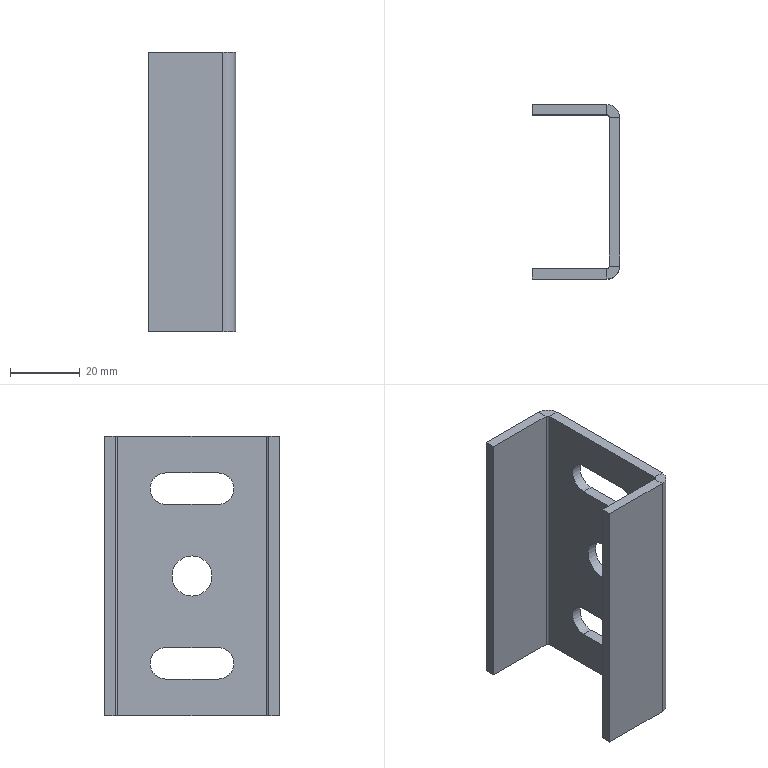Part | SolidWorks | features EdgeFlange 1, FlatPattern 1, SMBaseFlange 1, SheetMetal 1 | 1 solid | 32 faces | box 25 x 50 x 80 mm | volume 20596 mm3 | plane 22 | cylinder 10 | commonest cylinder face diameters 9 x4 1.473 x2 7.473 x2 11.5 x2
STEP:
#1=CARTESIAN_POINT('',(-3.,-25.,-34.25));
#2=VERTEX_POINT('',#1);
#3=CARTESIAN_POINT('',(-3.,-25.,-45.75));
#4=VERTEX_POINT('',#3);
#5=CARTESIAN_POINT('',(-3.,-25.,-40.));
#6=DIRECTION('',(1.,0.,0.));
#7=DIRECTION('',(0.,0.,-1.));
#8=AXIS2_PLACEMENT_3D('',#5,#6,#7);
#9=CIRCLE('',#8,5.75);
#10=EDGE_CURVE('',#2,#4,#9,.T.);
#11=ORIENTED_EDGE('',*,*,#10,.F.);
#12=CARTESIAN_POINT('',(0.,-25.,-34.25));
#13=VERTEX_POINT('',#12);
#14=CARTESIAN_POINT('',(-3.,-25.,-34.25));
#15=DIRECTION('',(1.,0.,0.));
#16=VECTOR('',#15,1000.);
#17=LINE('',#14,#16);
#18=EDGE_CURVE('',#2,#13,#17,.T.);
#19=ORIENTED_EDGE('',*,*,#18,.T.);
#20=CARTESIAN_POINT('',(0.,-25.,-45.75));
#21=VERTEX_POINT('',#20);
#22=CARTESIAN_POINT('',(0.,-25.,-40.));
#23=DIRECTION('',(1.,0.,0.));
#24=DIRECTION('',(0.,0.,-1.));
#25=AXIS2_PLACEMENT_3D('',#22,#23,#24);
#26=CIRCLE('',#25,5.75);
#27=EDGE_CURVE('',#13,#21,#26,.T.);
#28=ORIENTED_EDGE('',*,*,#27,.T.);
#29=CARTESIAN_POINT('',(-3.,-25.,-45.75));
#30=DIRECTION('',(1.,0.,0.));
#31=VECTOR('',#30,1000.);
#32=LINE('',#29,#31);
#33=EDGE_CURVE('',#4,#21,#32,.T.);
#34=ORIENTED_EDGE('',*,*,#33,.F.);
#35=EDGE_LOOP('',(#11,#19,#28,#34));
#36=FACE_OUTER_BOUND('',#35,.T.);
#37=CARTESIAN_POINT('',(-3.,-25.,-40.));
#38=DIRECTION('',(1.,0.,0.));
#39=DIRECTION('',(0.,0.,-1.));
#40=AXIS2_PLACEMENT_3D('',#37,#38,#39);
#41=CYLINDRICAL_SURFACE('',#40,5.75);
#42=ADVANCED_FACE('',(#36),#41,.F.);
#43=CARTESIAN_POINT('',(-3.,-32.5,-69.5));
#44=VERTEX_POINT('',#43);
#45=CARTESIAN_POINT('',(-3.,-17.5,-69.5));
#46=VERTEX_POINT('',#45);
#47=CARTESIAN_POINT('',(-3.,-17.5,-69.5));
#48=DIRECTION('',(0.,1.,0.));
#49=VECTOR('',#48,1000.);
#50=LINE('',#47,#49);
#51=EDGE_CURVE('',#44,#46,#50,.T.);
#52=ORIENTED_EDGE('',*,*,#51,.T.);
#53=CARTESIAN_POINT('',(-3.,-17.5,-60.5));
#54=VERTEX_POINT('',#53);
#55=CARTESIAN_POINT('',(-3.,-17.5,-65.));
#56=DIRECTION('',(1.,0.,0.));
#57=DIRECTION('',(0.,0.,-1.));
#58=AXIS2_PLACEMENT_3D('',#55,#56,#57);
#59=CIRCLE('',#58,4.5);
#60=EDGE_CURVE('',#46,#54,#59,.T.);
#61=ORIENTED_EDGE('',*,*,#60,.T.);
#62=CARTESIAN_POINT('',(-3.,-32.5,-60.5));
#63=VERTEX_POINT('',#62);
#64=CARTESIAN_POINT('',(-3.,-17.5,-60.5));
#65=DIRECTION('',(0.,-1.,0.));
#66=VECTOR('',#65,1000.);
#67=LINE('',#64,#66);
#68=EDGE_CURVE('',#54,#63,#67,.T.);
#69=ORIENTED_EDGE('',*,*,#68,.T.);
#70=CARTESIAN_POINT('',(-3.,-32.5,-65.));
#71=DIRECTION('',(1.,0.,0.));
#72=DIRECTION('',(0.,0.,-1.));
#73=AXIS2_PLACEMENT_3D('',#70,#71,#72);
#74=CIRCLE('',#73,4.5);
#75=EDGE_CURVE('',#63,#44,#74,.T.);
#76=ORIENTED_EDGE('',*,*,#75,.T.);
#77=EDGE_LOOP('',(#52,#61,#69,#76));
#78=FACE_BOUND('',#77,.T.);
#79=CARTESIAN_POINT('',(-3.,-32.5,-19.5));
#80=VERTEX_POINT('',#79);
#81=CARTESIAN_POINT('',(-3.,-17.5,-19.5));
#82=VERTEX_POINT('',#81);
#83=CARTESIAN_POINT('',(-3.,-17.5,-19.5));
#84=DIRECTION('',(0.,1.,0.));
#85=VECTOR('',#84,1000.);
#86=LINE('',#83,#85);
#87=EDGE_CURVE('',#80,#82,#86,.T.);
#88=ORIENTED_EDGE('',*,*,#87,.T.);
#89=CARTESIAN_POINT('',(-3.,-17.5,-10.5));
#90=VERTEX_POINT('',#89);
#91=CARTESIAN_POINT('',(-3.,-17.5,-15.));
#92=DIRECTION('',(1.,0.,0.));
#93=DIRECTION('',(0.,0.,-1.));
#94=AXIS2_PLACEMENT_3D('',#91,#92,#93);
#95=CIRCLE('',#94,4.5);
#96=EDGE_CURVE('',#82,#90,#95,.T.);
#97=ORIENTED_EDGE('',*,*,#96,.T.);
#98=CARTESIAN_POINT('',(-3.,-32.5,-10.5));
#99=VERTEX_POINT('',#98);
#100=CARTESIAN_POINT('',(-3.,-17.5,-10.5));
#101=DIRECTION('',(0.,-1.,0.));
#102=VECTOR('',#101,1000.);
#103=LINE('',#100,#102);
#104=EDGE_CURVE('',#90,#99,#103,.T.);
#105=ORIENTED_EDGE('',*,*,#104,.T.);
#106=CARTESIAN_POINT('',(-3.,-32.5,-15.));
#107=DIRECTION('',(1.,0.,0.));
#108=DIRECTION('',(0.,0.,-1.));
#109=AXIS2_PLACEMENT_3D('',#106,#107,#108);
#110=CIRCLE('',#109,4.5);
#111=EDGE_CURVE('',#99,#80,#110,.T.);
#112=ORIENTED_EDGE('',*,*,#111,.T.);
#113=EDGE_LOOP('',(#88,#97,#105,#112));
#114=FACE_BOUND('',#113,.T.);
#115=CARTESIAN_POINT('',(-3.,-25.,-40.));
#116=DIRECTION('',(1.,0.,0.));
#117=DIRECTION('',(0.,0.,-1.));
#118=AXIS2_PLACEMENT_3D('',#115,#116,#117);
#119=CIRCLE('',#118,5.75);
#120=EDGE_CURVE('',#4,#2,#119,.T.);
#121=ORIENTED_EDGE('',*,*,#120,.T.);
#122=ORIENTED_EDGE('',*,*,#10,.T.);
#123=EDGE_LOOP('',(#121,#122));
#124=FACE_BOUND('',#123,.T.);
#125=CARTESIAN_POINT('',(-3.,-46.263,0.));
#126=VERTEX_POINT('',#125);
#127=CARTESIAN_POINT('',(-3.,-46.263,-80.));
#128=VERTEX_POINT('',#127);
#129=CARTESIAN_POINT('',(-3.,-46.263,0.));
#130=DIRECTION('',(0.,0.,-1.));
#131=VECTOR('',#130,1000.);
#132=LINE('',#129,#131);
#133=EDGE_CURVE('',#126,#128,#132,.T.);
#134=ORIENTED_EDGE('',*,*,#133,.F.);
#135=CARTESIAN_POINT('',(-3.,-3.737,0.));
#136=VERTEX_POINT('',#135);
#137=CARTESIAN_POINT('',(-3.,0.,0.));
#138=DIRECTION('',(0.,-1.,0.));
#139=VECTOR('',#138,1000.);
#140=LINE('',#137,#139);
#141=EDGE_CURVE('',#136,#126,#140,.T.);
#142=ORIENTED_EDGE('',*,*,#141,.F.);
#143=CARTESIAN_POINT('',(-3.,-3.737,-80.));
#144=VERTEX_POINT('',#143);
#145=CARTESIAN_POINT('',(-3.,-3.737,-80.));
#146=DIRECTION('',(0.,0.,1.));
#147=VECTOR('',#146,1000.);
#148=LINE('',#145,#147);
#149=EDGE_CURVE('',#144,#136,#148,.T.);
#150=ORIENTED_EDGE('',*,*,#149,.F.);
#151=CARTESIAN_POINT('',(-3.,0.,-80.));
#152=DIRECTION('',(0.,1.,0.));
#153=VECTOR('',#152,1000.);
#154=LINE('',#151,#153);
#155=EDGE_CURVE('',#128,#144,#154,.T.);
#156=ORIENTED_EDGE('',*,*,#155,.F.);
#157=EDGE_LOOP('',(#134,#142,#150,#156));
#158=FACE_OUTER_BOUND('',#157,.T.);
#159=CARTESIAN_POINT('',(-3.,0.,0.));
#160=DIRECTION('',(1.,0.,0.));
#161=DIRECTION('',(0.,0.,-1.));
#162=AXIS2_PLACEMENT_3D('',#159,#160,#161);
#163=PLANE('',#162);
#164=ADVANCED_FACE('',(#78,#114,#124,#158),#163,.F.);
#165=CARTESIAN_POINT('',(0.,-17.5,-69.5));
#166=VERTEX_POINT('',#165);
#167=CARTESIAN_POINT('',(0.,-17.5,-60.5));
#168=VERTEX_POINT('',#167);
#169=CARTESIAN_POINT('',(0.,-17.5,-65.));
#170=DIRECTION('',(1.,0.,0.));
#171=DIRECTION('',(0.,0.,-1.));
#172=AXIS2_PLACEMENT_3D('',#169,#170,#171);
#173=CIRCLE('',#172,4.5);
#174=EDGE_CURVE('',#166,#168,#173,.T.);
#175=ORIENTED_EDGE('',*,*,#174,.F.);
#176=CARTESIAN_POINT('',(0.,-32.5,-69.5));
#177=VERTEX_POINT('',#176);
#178=CARTESIAN_POINT('',(0.,-17.5,-69.5));
#179=DIRECTION('',(0.,1.,0.));
#180=VECTOR('',#179,1000.);
#181=LINE('',#178,#180);
#182=EDGE_CURVE('',#177,#166,#181,.T.);
#183=ORIENTED_EDGE('',*,*,#182,.F.);
#184=CARTESIAN_POINT('',(0.,-32.5,-60.5));
#185=VERTEX_POINT('',#184);
#186=CARTESIAN_POINT('',(0.,-32.5,-65.));
#187=DIRECTION('',(1.,0.,0.));
#188=DIRECTION('',(0.,0.,-1.));
#189=AXIS2_PLACEMENT_3D('',#186,#187,#188);
#190=CIRCLE('',#189,4.5);
#191=EDGE_CURVE('',#185,#177,#190,.T.);
#192=ORIENTED_EDGE('',*,*,#191,.F.);
#193=CARTESIAN_POINT('',(0.,-17.5,-60.5));
#194=DIRECTION('',(0.,-1.,0.));
#195=VECTOR('',#194,1000.);
#196=LINE('',#193,#195);
#197=EDGE_CURVE('',#168,#185,#196,.T.);
#198=ORIENTED_EDGE('',*,*,#197,.F.);
#199=EDGE_LOOP('',(#175,#183,#192,#198));
#200=FACE_BOUND('',#199,.T.);
#201=CARTESIAN_POINT('',(0.,-17.5,-19.5));
#202=VERTEX_POINT('',#201);
#203=CARTESIAN_POINT('',(0.,-17.5,-10.5));
#204=VERTEX_POINT('',#203);
#205=CARTESIAN_POINT('',(0.,-17.5,-15.));
#206=DIRECTION('',(1.,0.,0.));
#207=DIRECTION('',(0.,0.,-1.));
#208=AXIS2_PLACEMENT_3D('',#205,#206,#207);
#209=CIRCLE('',#208,4.5);
#210=EDGE_CURVE('',#202,#204,#209,.T.);
#211=ORIENTED_EDGE('',*,*,#210,.F.);
#212=CARTESIAN_POINT('',(0.,-32.5,-19.5));
#213=VERTEX_POINT('',#212);
#214=CARTESIAN_POINT('',(0.,-17.5,-19.5));
#215=DIRECTION('',(0.,1.,0.));
#216=VECTOR('',#215,1000.);
#217=LINE('',#214,#216);
#218=EDGE_CURVE('',#213,#202,#217,.T.);
#219=ORIENTED_EDGE('',*,*,#218,.F.);
#220=CARTESIAN_POINT('',(0.,-32.5,-10.5));
#221=VERTEX_POINT('',#220);
#222=CARTESIAN_POINT('',(0.,-32.5,-15.));
#223=DIRECTION('',(1.,0.,0.));
#224=DIRECTION('',(0.,0.,-1.));
#225=AXIS2_PLACEMENT_3D('',#222,#223,#224);
#226=CIRCLE('',#225,4.5);
#227=EDGE_CURVE('',#221,#213,#226,.T.);
#228=ORIENTED_EDGE('',*,*,#227,.F.);
#229=CARTESIAN_POINT('',(0.,-17.5,-10.5));
#230=DIRECTION('',(0.,-1.,0.));
#231=VECTOR('',#230,1000.);
#232=LINE('',#229,#231);
#233=EDGE_CURVE('',#204,#221,#232,.T.);
#234=ORIENTED_EDGE('',*,*,#233,.F.);
#235=EDGE_LOOP('',(#211,#219,#228,#234));
#236=FACE_BOUND('',#235,.T.);
#237=CARTESIAN_POINT('',(0.,-25.,-40.));
#238=DIRECTION('',(1.,0.,0.));
#239=DIRECTION('',(0.,0.,-1.));
#240=AXIS2_PLACEMENT_3D('',#237,#238,#239);
#241=CIRCLE('',#240,5.75);
#242=EDGE_CURVE('',#21,#13,#241,.T.);
#243=ORIENTED_EDGE('',*,*,#242,.F.);
#244=ORIENTED_EDGE('',*,*,#27,.F.);
#245=EDGE_LOOP('',(#243,#244));
#246=FACE_BOUND('',#245,.T.);
#247=CARTESIAN_POINT('',(0.,-3.737,0.));
#248=VERTEX_POINT('',#247);
#249=CARTESIAN_POINT('',(0.,-46.263,0.));
#250=VERTEX_POINT('',#249);
#251=CARTESIAN_POINT('',(0.,0.,0.));
#252=DIRECTION('',(0.,-1.,0.));
#253=VECTOR('',#252,1000.);
#254=LINE('',#251,#253);
#255=EDGE_CURVE('',#248,#250,#254,.T.);
#256=ORIENTED_EDGE('',*,*,#255,.T.);
#257=CARTESIAN_POINT('',(0.,-46.263,-80.));
#258=VERTEX_POINT('',#257);
#259=CARTESIAN_POINT('',(0.,-46.263,0.));
#260=DIRECTION('',(0.,0.,-1.));
#261=VECTOR('',#260,1000.);
#262=LINE('',#259,#261);
#263=EDGE_CURVE('',#250,#258,#262,.T.);
#264=ORIENTED_EDGE('',*,*,#263,.T.);
#265=CARTESIAN_POINT('',(0.,-3.737,-80.));
#266=VERTEX_POINT('',#265);
#267=CARTESIAN_POINT('',(0.,0.,-80.));
#268=DIRECTION('',(0.,1.,0.));
#269=VECTOR('',#268,1000.);
#270=LINE('',#267,#269);
#271=EDGE_CURVE('',#258,#266,#270,.T.);
#272=ORIENTED_EDGE('',*,*,#271,.T.);
#273=CARTESIAN_POINT('',(0.,-3.737,-80.));
#274=DIRECTION('',(0.,0.,1.));
#275=VECTOR('',#274,1000.);
#276=LINE('',#273,#275);
#277=EDGE_CURVE('',#266,#248,#276,.T.);
#278=ORIENTED_EDGE('',*,*,#277,.T.);
#279=EDGE_LOOP('',(#256,#264,#272,#278));
#280=FACE_OUTER_BOUND('',#279,.T.);
#281=CARTESIAN_POINT('',(0.,0.,0.));
#282=DIRECTION('',(1.,0.,0.));
#283=DIRECTION('',(0.,0.,-1.));
#284=AXIS2_PLACEMENT_3D('',#281,#282,#283);
#285=PLANE('',#284);
#286=ADVANCED_FACE('',(#200,#236,#246,#280),#285,.T.);
#287=ORIENTED_EDGE('',*,*,#141,.T.);
#288=CARTESIAN_POINT('',(-3.,-46.263,0.));
#289=DIRECTION('',(1.,0.,0.));
#290=VECTOR('',#289,1000.);
#291=LINE('',#288,#290);
#292=EDGE_CURVE('',#126,#250,#291,.T.);
#293=ORIENTED_EDGE('',*,*,#292,.T.);
#294=ORIENTED_EDGE('',*,*,#255,.F.);
#295=CARTESIAN_POINT('',(-3.,-3.737,0.));
#296=DIRECTION('',(1.,0.,0.));
#297=VECTOR('',#296,1000.);
#298=LINE('',#295,#297);
#299=EDGE_CURVE('',#136,#248,#298,.T.);
#300=ORIENTED_EDGE('',*,*,#299,.F.);
#301=EDGE_LOOP('',(#287,#293,#294,#300));
#302=FACE_OUTER_BOUND('',#301,.T.);
#303=CARTESIAN_POINT('',(-3.,0.,0.));
#304=DIRECTION('',(0.,0.,1.));
#305=DIRECTION('',(0.,-1.,0.));
#306=AXIS2_PLACEMENT_3D('',#303,#304,#305);
#307=PLANE('',#306);
#308=ADVANCED_FACE('',(#302),#307,.T.);
#309=CARTESIAN_POINT('',(-3.,-46.263,-80.));
#310=DIRECTION('',(1.,0.,0.));
#311=VECTOR('',#310,1000.);
#312=LINE('',#309,#311);
#313=EDGE_CURVE('',#128,#258,#312,.T.);
#314=ORIENTED_EDGE('',*,*,#313,.F.);
#315=ORIENTED_EDGE('',*,*,#155,.T.);
#316=CARTESIAN_POINT('',(-3.,-3.737,-80.));
#317=DIRECTION('',(1.,0.,0.));
#318=VECTOR('',#317,1000.);
#319=LINE('',#316,#318);
#320=EDGE_CURVE('',#144,#266,#319,.T.);
#321=ORIENTED_EDGE('',*,*,#320,.T.);
#322=ORIENTED_EDGE('',*,*,#271,.F.);
#323=EDGE_LOOP('',(#314,#315,#321,#322));
#324=FACE_OUTER_BOUND('',#323,.T.);
#325=CARTESIAN_POINT('',(-3.,0.,-80.));
#326=DIRECTION('',(0.,0.,-1.));
#327=DIRECTION('',(-1.,0.,0.));
#328=AXIS2_PLACEMENT_3D('',#325,#326,#327);
#329=PLANE('',#328);
#330=ADVANCED_FACE('',(#324),#329,.T.);
#331=ORIENTED_EDGE('',*,*,#18,.F.);
#332=ORIENTED_EDGE('',*,*,#120,.F.);
#333=ORIENTED_EDGE('',*,*,#33,.T.);
#334=ORIENTED_EDGE('',*,*,#242,.T.);
#335=EDGE_LOOP('',(#331,#332,#333,#334));
#336=FACE_OUTER_BOUND('',#335,.T.);
#337=CARTESIAN_POINT('',(-3.,-25.,-40.));
#338=DIRECTION('',(1.,0.,0.));
#339=DIRECTION('',(0.,0.,-1.));
#340=AXIS2_PLACEMENT_3D('',#337,#338,#339);
#341=CYLINDRICAL_SURFACE('',#340,5.75);
#342=ADVANCED_FACE('',(#336),#341,.F.);
#343=ORIENTED_EDGE('',*,*,#210,.T.);
#344=CARTESIAN_POINT('',(-3.,-17.5,-10.5));
#345=DIRECTION('',(1.,0.,0.));
#346=VECTOR('',#345,1000.);
#347=LINE('',#344,#346);
#348=EDGE_CURVE('',#90,#204,#347,.T.);
#349=ORIENTED_EDGE('',*,*,#348,.F.);
#350=ORIENTED_EDGE('',*,*,#96,.F.);
#351=CARTESIAN_POINT('',(-3.,-17.5,-19.5));
#352=DIRECTION('',(1.,0.,0.));
#353=VECTOR('',#352,1000.);
#354=LINE('',#351,#353);
#355=EDGE_CURVE('',#82,#202,#354,.T.);
#356=ORIENTED_EDGE('',*,*,#355,.T.);
#357=EDGE_LOOP('',(#343,#349,#350,#356));
#358=FACE_OUTER_BOUND('',#357,.T.);
#359=CARTESIAN_POINT('',(-3.,-17.5,-15.));
#360=DIRECTION('',(1.,0.,0.));
#361=DIRECTION('',(0.,0.,-1.));
#362=AXIS2_PLACEMENT_3D('',#359,#360,#361);
#363=CYLINDRICAL_SURFACE('',#362,4.5);
#364=ADVANCED_FACE('',(#358),#363,.F.);
#365=ORIENTED_EDGE('',*,*,#218,.T.);
#366=ORIENTED_EDGE('',*,*,#355,.F.);
#367=ORIENTED_EDGE('',*,*,#87,.F.);
#368=CARTESIAN_POINT('',(-3.,-32.5,-19.5));
#369=DIRECTION('',(1.,0.,0.));
#370=VECTOR('',#369,1000.);
#371=LINE('',#368,#370);
#372=EDGE_CURVE('',#80,#213,#371,.T.);
#373=ORIENTED_EDGE('',*,*,#372,.T.);
#374=EDGE_LOOP('',(#365,#366,#367,#373));
#375=FACE_OUTER_BOUND('',#374,.T.);
#376=CARTESIAN_POINT('',(-3.,-17.5,-19.5));
#377=DIRECTION('',(0.,0.,-1.));
#378=DIRECTION('',(-1.,0.,0.));
#379=AXIS2_PLACEMENT_3D('',#376,#377,#378);
#380=PLANE('',#379);
#381=ADVANCED_FACE('',(#375),#380,.F.);
#382=ORIENTED_EDGE('',*,*,#227,.T.);
#383=ORIENTED_EDGE('',*,*,#372,.F.);
#384=ORIENTED_EDGE('',*,*,#111,.F.);
#385=CARTESIAN_POINT('',(-3.,-32.5,-10.5));
#386=DIRECTION('',(1.,0.,0.));
#387=VECTOR('',#386,1000.);
#388=LINE('',#385,#387);
#389=EDGE_CURVE('',#99,#221,#388,.T.);
#390=ORIENTED_EDGE('',*,*,#389,.T.);
#391=EDGE_LOOP('',(#382,#383,#384,#390));
#392=FACE_OUTER_BOUND('',#391,.T.);
#393=CARTESIAN_POINT('',(-3.,-32.5,-15.));
#394=DIRECTION('',(1.,0.,0.));
#395=DIRECTION('',(0.,0.,-1.));
#396=AXIS2_PLACEMENT_3D('',#393,#394,#395);
#397=CYLINDRICAL_SURFACE('',#396,4.5);
#398=ADVANCED_FACE('',(#392),#397,.F.);
#399=ORIENTED_EDGE('',*,*,#233,.T.);
#400=ORIENTED_EDGE('',*,*,#389,.F.);
#401=ORIENTED_EDGE('',*,*,#104,.F.);
#402=ORIENTED_EDGE('',*,*,#348,.T.);
#403=EDGE_LOOP('',(#399,#400,#401,#402));
#404=FACE_OUTER_BOUND('',#403,.T.);
#405=CARTESIAN_POINT('',(-3.,-17.5,-10.5));
#406=DIRECTION('',(0.,0.,1.));
#407=DIRECTION('',(1.,0.,0.));
#408=AXIS2_PLACEMENT_3D('',#405,#406,#407);
#409=PLANE('',#408);
#410=ADVANCED_FACE('',(#404),#409,.F.);
#411=ORIENTED_EDGE('',*,*,#174,.T.);
#412=CARTESIAN_POINT('',(-3.,-17.5,-60.5));
#413=DIRECTION('',(1.,0.,0.));
#414=VECTOR('',#413,1000.);
#415=LINE('',#412,#414);
#416=EDGE_CURVE('',#54,#168,#415,.T.);
#417=ORIENTED_EDGE('',*,*,#416,.F.);
#418=ORIENTED_EDGE('',*,*,#60,.F.);
#419=CARTESIAN_POINT('',(-3.,-17.5,-69.5));
#420=DIRECTION('',(1.,0.,0.));
#421=VECTOR('',#420,1000.);
#422=LINE('',#419,#421);
#423=EDGE_CURVE('',#46,#166,#422,.T.);
#424=ORIENTED_EDGE('',*,*,#423,.T.);
#425=EDGE_LOOP('',(#411,#417,#418,#424));
#426=FACE_OUTER_BOUND('',#425,.T.);
#427=CARTESIAN_POINT('',(-3.,-17.5,-65.));
#428=DIRECTION('',(1.,0.,0.));
#429=DIRECTION('',(0.,0.,-1.));
#430=AXIS2_PLACEMENT_3D('',#427,#428,#429);
#431=CYLINDRICAL_SURFACE('',#430,4.5);
#432=ADVANCED_FACE('',(#426),#431,.F.);
#433=ORIENTED_EDGE('',*,*,#182,.T.);
#434=ORIENTED_EDGE('',*,*,#423,.F.);
#435=ORIENTED_EDGE('',*,*,#51,.F.);
#436=CARTESIAN_POINT('',(-3.,-32.5,-69.5));
#437=DIRECTION('',(1.,0.,0.));
#438=VECTOR('',#437,1000.);
#439=LINE('',#436,#438);
#440=EDGE_CURVE('',#44,#177,#439,.T.);
#441=ORIENTED_EDGE('',*,*,#440,.T.);
#442=EDGE_LOOP('',(#433,#434,#435,#441));
#443=FACE_OUTER_BOUND('',#442,.T.);
#444=CARTESIAN_POINT('',(-3.,-17.5,-69.5));
#445=DIRECTION('',(0.,0.,-1.));
#446=DIRECTION('',(0.,1.,0.));
#447=AXIS2_PLACEMENT_3D('',#444,#445,#446);
#448=PLANE('',#447);
#449=ADVANCED_FACE('',(#443),#448,.F.);
#450=ORIENTED_EDGE('',*,*,#191,.T.);
#451=ORIENTED_EDGE('',*,*,#440,.F.);
#452=ORIENTED_EDGE('',*,*,#75,.F.);
#453=CARTESIAN_POINT('',(-3.,-32.5,-60.5));
#454=DIRECTION('',(1.,0.,0.));
#455=VECTOR('',#454,1000.);
#456=LINE('',#453,#455);
#457=EDGE_CURVE('',#63,#185,#456,.T.);
#458=ORIENTED_EDGE('',*,*,#457,.T.);
#459=EDGE_LOOP('',(#450,#451,#452,#458));
#460=FACE_OUTER_BOUND('',#459,.T.);
#461=CARTESIAN_POINT('',(-3.,-32.5,-65.));
#462=DIRECTION('',(1.,0.,0.));
#463=DIRECTION('',(0.,0.,-1.));
#464=AXIS2_PLACEMENT_3D('',#461,#462,#463);
#465=CYLINDRICAL_SURFACE('',#464,4.5);
#466=ADVANCED_FACE('',(#460),#465,.F.);
#467=ORIENTED_EDGE('',*,*,#197,.T.);
#468=ORIENTED_EDGE('',*,*,#457,.F.);
#469=ORIENTED_EDGE('',*,*,#68,.F.);
#470=ORIENTED_EDGE('',*,*,#416,.T.);
#471=EDGE_LOOP('',(#467,#468,#469,#470));
#472=FACE_OUTER_BOUND('',#471,.T.);
#473=CARTESIAN_POINT('',(-3.,-17.5,-60.5));
#474=DIRECTION('',(0.,0.,1.));
#475=DIRECTION('',(0.,-1.,0.));
#476=AXIS2_PLACEMENT_3D('',#473,#474,#475);
#477=PLANE('',#476);
#478=ADVANCED_FACE('',(#472),#477,.F.);
#479=CARTESIAN_POINT('',(-3.737,-3.,0.));
#480=VERTEX_POINT('',#479);
#481=CARTESIAN_POINT('',(-3.737,0.,0.));
#482=VERTEX_POINT('',#481);
#483=CARTESIAN_POINT('',(-3.737,0.,0.));
#484=DIRECTION('',(0.,1.,0.));
#485=VECTOR('',#484,1000.);
#486=LINE('',#483,#485);
#487=EDGE_CURVE('',#480,#482,#486,.T.);
#488=ORIENTED_EDGE('',*,*,#487,.F.);
#489=CARTESIAN_POINT('',(-3.737,-3.737,0.));
#490=DIRECTION('',(0.,0.,1.));
#491=DIRECTION('',(-1.,0.,0.));
#492=AXIS2_PLACEMENT_3D('',#489,#490,#491);
#493=CIRCLE('',#492,0.7366);
#494=EDGE_CURVE('',#136,#480,#493,.T.);
#495=ORIENTED_EDGE('',*,*,#494,.F.);
#496=ORIENTED_EDGE('',*,*,#299,.T.);
#497=CARTESIAN_POINT('',(-3.737,-3.737,0.));
#498=DIRECTION('',(0.,0.,1.));
#499=DIRECTION('',(-1.,0.,0.));
#500=AXIS2_PLACEMENT_3D('',#497,#498,#499);
#501=CIRCLE('',#500,3.737);
#502=EDGE_CURVE('',#248,#482,#501,.T.);
#503=ORIENTED_EDGE('',*,*,#502,.T.);
#504=EDGE_LOOP('',(#488,#495,#496,#503));
#505=FACE_OUTER_BOUND('',#504,.T.);
#506=CARTESIAN_POINT('',(-3.737,-3.737,0.));
#507=DIRECTION('',(0.,0.,1.));
#508=DIRECTION('',(1.,0.,0.));
#509=AXIS2_PLACEMENT_3D('',#506,#507,#508);
#510=PLANE('',#509);
#511=ADVANCED_FACE('',(#505),#510,.T.);
#512=CARTESIAN_POINT('',(-3.737,-3.,-80.));
#513=VERTEX_POINT('',#512);
#514=CARTESIAN_POINT('',(-3.737,-3.737,-80.));
#515=DIRECTION('',(0.,0.,-1.));
#516=DIRECTION('',(-1.,0.,0.));
#517=AXIS2_PLACEMENT_3D('',#514,#515,#516);
#518=CIRCLE('',#517,0.7366);
#519=EDGE_CURVE('',#513,#144,#518,.T.);
#520=ORIENTED_EDGE('',*,*,#519,.F.);
#521=CARTESIAN_POINT('',(-3.737,0.,-80.));
#522=VERTEX_POINT('',#521);
#523=CARTESIAN_POINT('',(-3.737,-3.,-80.));
#524=DIRECTION('',(0.,1.,0.));
#525=VECTOR('',#524,1000.);
#526=LINE('',#523,#525);
#527=EDGE_CURVE('',#513,#522,#526,.T.);
#528=ORIENTED_EDGE('',*,*,#527,.T.);
#529=CARTESIAN_POINT('',(-3.737,-3.737,-80.));
#530=DIRECTION('',(0.,0.,-1.));
#531=DIRECTION('',(-1.,0.,0.));
#532=AXIS2_PLACEMENT_3D('',#529,#530,#531);
#533=CIRCLE('',#532,3.737);
#534=EDGE_CURVE('',#522,#266,#533,.T.);
#535=ORIENTED_EDGE('',*,*,#534,.T.);
#536=ORIENTED_EDGE('',*,*,#320,.F.);
#537=EDGE_LOOP('',(#520,#528,#535,#536));
#538=FACE_OUTER_BOUND('',#537,.T.);
#539=CARTESIAN_POINT('',(-3.737,-3.737,-80.));
#540=DIRECTION('',(0.,0.,1.));
#541=DIRECTION('',(1.,0.,0.));
#542=AXIS2_PLACEMENT_3D('',#539,#540,#541);
#543=PLANE('',#542);
#544=ADVANCED_FACE('',(#538),#543,.F.);
#545=ORIENTED_EDGE('',*,*,#277,.F.);
#546=ORIENTED_EDGE('',*,*,#534,.F.);
#547=CARTESIAN_POINT('',(-3.737,0.,0.));
#548=DIRECTION('',(0.,0.,1.));
#549=VECTOR('',#548,1000.);
#550=LINE('',#547,#549);
#551=EDGE_CURVE('',#522,#482,#550,.T.);
#552=ORIENTED_EDGE('',*,*,#551,.T.);
#553=ORIENTED_EDGE('',*,*,#502,.F.);
#554=EDGE_LOOP('',(#545,#546,#552,#553));
#555=FACE_OUTER_BOUND('',#554,.T.);
#556=CARTESIAN_POINT('',(-3.737,-3.737,-80.));
#557=DIRECTION('',(0.,0.,-1.));
#558=DIRECTION('',(0.,1.,0.));
#559=AXIS2_PLACEMENT_3D('',#556,#557,#558);
#560=CYLINDRICAL_SURFACE('',#559,3.737);
#561=ADVANCED_FACE('',(#555),#560,.T.);
#562=ORIENTED_EDGE('',*,*,#149,.T.);
#563=ORIENTED_EDGE('',*,*,#494,.T.);
#564=CARTESIAN_POINT('',(-3.737,-3.,0.));
#565=DIRECTION('',(0.,0.,-1.));
#566=VECTOR('',#565,1000.);
#567=LINE('',#564,#566);
#568=EDGE_CURVE('',#480,#513,#567,.T.);
#569=ORIENTED_EDGE('',*,*,#568,.T.);
#570=ORIENTED_EDGE('',*,*,#519,.T.);
#571=EDGE_LOOP('',(#562,#563,#569,#570));
#572=FACE_OUTER_BOUND('',#571,.T.);
#573=CARTESIAN_POINT('',(-3.737,-3.737,-80.));
#574=DIRECTION('',(0.,0.,-1.));
#575=DIRECTION('',(0.,1.,0.));
#576=AXIS2_PLACEMENT_3D('',#573,#574,#575);
#577=CYLINDRICAL_SURFACE('',#576,0.7366);
#578=ADVANCED_FACE('',(#572),#577,.F.);
#579=ORIENTED_EDGE('',*,*,#527,.F.);
#580=CARTESIAN_POINT('',(-25.,-3.,-80.));
#581=VERTEX_POINT('',#580);
#582=CARTESIAN_POINT('',(-25.,-3.,-80.));
#583=DIRECTION('',(-1.,0.,0.));
#584=VECTOR('',#583,1000.);
#585=LINE('',#582,#584);
#586=EDGE_CURVE('',#513,#581,#585,.T.);
#587=ORIENTED_EDGE('',*,*,#586,.T.);
#588=CARTESIAN_POINT('',(-25.,0.,-80.));
#589=VERTEX_POINT('',#588);
#590=CARTESIAN_POINT('',(-25.,0.,-80.));
#591=DIRECTION('',(0.,-1.,0.));
#592=VECTOR('',#591,1000.);
#593=LINE('',#590,#592);
#594=EDGE_CURVE('',#589,#581,#593,.T.);
#595=ORIENTED_EDGE('',*,*,#594,.F.);
#596=CARTESIAN_POINT('',(0.,0.,-80.));
#597=DIRECTION('',(-1.,0.,0.));
#598=VECTOR('',#597,1000.);
#599=LINE('',#596,#598);
#600=EDGE_CURVE('',#522,#589,#599,.T.);
#601=ORIENTED_EDGE('',*,*,#600,.F.);
#602=EDGE_LOOP('',(#579,#587,#595,#601));
#603=FACE_OUTER_BOUND('',#602,.T.);
#604=CARTESIAN_POINT('',(-25.,0.,-80.));
#605=DIRECTION('',(0.,0.,1.));
#606=DIRECTION('',(1.,0.,0.));
#607=AXIS2_PLACEMENT_3D('',#604,#605,#606);
#608=PLANE('',#607);
#609=ADVANCED_FACE('',(#603),#608,.F.);
#610=ORIENTED_EDGE('',*,*,#487,.T.);
#611=CARTESIAN_POINT('',(-25.,0.,0.));
#612=VERTEX_POINT('',#611);
#613=CARTESIAN_POINT('',(0.,0.,0.));
#614=DIRECTION('',(1.,0.,0.));
#615=VECTOR('',#614,1000.);
#616=LINE('',#613,#615);
#617=EDGE_CURVE('',#612,#482,#616,.T.);
#618=ORIENTED_EDGE('',*,*,#617,.F.);
#619=CARTESIAN_POINT('',(-25.,-3.,0.));
#620=VERTEX_POINT('',#619);
#621=CARTESIAN_POINT('',(-25.,0.,0.));
#622=DIRECTION('',(0.,-1.,0.));
#623=VECTOR('',#622,1000.);
#624=LINE('',#621,#623);
#625=EDGE_CURVE('',#612,#620,#624,.T.);
#626=ORIENTED_EDGE('',*,*,#625,.T.);
#627=CARTESIAN_POINT('',(-3.,-3.,0.));
#628=DIRECTION('',(1.,0.,0.));
#629=VECTOR('',#628,1000.);
#630=LINE('',#627,#629);
#631=EDGE_CURVE('',#620,#480,#630,.T.);
#632=ORIENTED_EDGE('',*,*,#631,.T.);
#633=EDGE_LOOP('',(#610,#618,#626,#632));
#634=FACE_OUTER_BOUND('',#633,.T.);
#635=CARTESIAN_POINT('',(-3.,0.,0.));
#636=DIRECTION('',(0.,0.,-1.));
#637=DIRECTION('',(-1.,0.,0.));
#638=AXIS2_PLACEMENT_3D('',#635,#636,#637);
#639=PLANE('',#638);
#640=ADVANCED_FACE('',(#634),#639,.F.);
#641=ORIENTED_EDGE('',*,*,#551,.F.);
#642=ORIENTED_EDGE('',*,*,#600,.T.);
#643=CARTESIAN_POINT('',(-25.,0.,0.));
#644=DIRECTION('',(0.,0.,1.));
#645=VECTOR('',#644,1000.);
#646=LINE('',#643,#645);
#647=EDGE_CURVE('',#589,#612,#646,.T.);
#648=ORIENTED_EDGE('',*,*,#647,.T.);
#649=ORIENTED_EDGE('',*,*,#617,.T.);
#650=EDGE_LOOP('',(#641,#642,#648,#649));
#651=FACE_OUTER_BOUND('',#650,.T.);
#652=CARTESIAN_POINT('',(0.,0.,0.));
#653=DIRECTION('',(0.,-1.,0.));
#654=DIRECTION('',(1.,0.,0.));
#655=AXIS2_PLACEMENT_3D('',#652,#653,#654);
#656=PLANE('',#655);
#657=ADVANCED_FACE('',(#651),#656,.F.);
#658=ORIENTED_EDGE('',*,*,#586,.F.);
#659=ORIENTED_EDGE('',*,*,#568,.F.);
#660=ORIENTED_EDGE('',*,*,#631,.F.);
#661=CARTESIAN_POINT('',(-25.,-3.,0.));
#662=DIRECTION('',(0.,0.,1.));
#663=VECTOR('',#662,1000.);
#664=LINE('',#661,#663);
#665=EDGE_CURVE('',#581,#620,#664,.T.);
#666=ORIENTED_EDGE('',*,*,#665,.F.);
#667=EDGE_LOOP('',(#658,#659,#660,#666));
#668=FACE_OUTER_BOUND('',#667,.T.);
#669=CARTESIAN_POINT('',(0.,-3.,0.));
#670=DIRECTION('',(0.,-1.,0.));
#671=DIRECTION('',(1.,0.,0.));
#672=AXIS2_PLACEMENT_3D('',#669,#670,#671);
#673=PLANE('',#672);
#674=ADVANCED_FACE('',(#668),#673,.T.);
#675=ORIENTED_EDGE('',*,*,#665,.T.);
#676=ORIENTED_EDGE('',*,*,#625,.F.);
#677=ORIENTED_EDGE('',*,*,#647,.F.);
#678=ORIENTED_EDGE('',*,*,#594,.T.);
#679=EDGE_LOOP('',(#675,#676,#677,#678));
#680=FACE_OUTER_BOUND('',#679,.T.);
#681=CARTESIAN_POINT('',(-25.,0.,0.));
#682=DIRECTION('',(1.,0.,0.));
#683=DIRECTION('',(0.,1.,0.));
#684=AXIS2_PLACEMENT_3D('',#681,#682,#683);
#685=PLANE('',#684);
#686=ADVANCED_FACE('',(#680),#685,.F.);
#687=CARTESIAN_POINT('',(-3.737,-47.,-80.));
#688=VERTEX_POINT('',#687);
#689=CARTESIAN_POINT('',(-3.737,-50.,-80.));
#690=VERTEX_POINT('',#689);
#691=CARTESIAN_POINT('',(-3.737,-50.,-80.));
#692=DIRECTION('',(0.,-1.,0.));
#693=VECTOR('',#692,1000.);
#694=LINE('',#691,#693);
#695=EDGE_CURVE('',#688,#690,#694,.T.);
#696=ORIENTED_EDGE('',*,*,#695,.F.);
#697=CARTESIAN_POINT('',(-3.737,-46.263,-80.));
#698=DIRECTION('',(0.,0.,-1.));
#699=DIRECTION('',(1.,0.,0.));
#700=AXIS2_PLACEMENT_3D('',#697,#698,#699);
#701=CIRCLE('',#700,0.7366);
#702=EDGE_CURVE('',#128,#688,#701,.T.);
#703=ORIENTED_EDGE('',*,*,#702,.F.);
#704=ORIENTED_EDGE('',*,*,#313,.T.);
#705=CARTESIAN_POINT('',(-3.737,-46.263,-80.));
#706=DIRECTION('',(0.,0.,-1.));
#707=DIRECTION('',(1.,0.,0.));
#708=AXIS2_PLACEMENT_3D('',#705,#706,#707);
#709=CIRCLE('',#708,3.737);
#710=EDGE_CURVE('',#258,#690,#709,.T.);
#711=ORIENTED_EDGE('',*,*,#710,.T.);
#712=EDGE_LOOP('',(#696,#703,#704,#711));
#713=FACE_OUTER_BOUND('',#712,.T.);
#714=CARTESIAN_POINT('',(-3.737,-46.263,-80.));
#715=DIRECTION('',(0.,0.,-1.));
#716=DIRECTION('',(-1.,0.,0.));
#717=AXIS2_PLACEMENT_3D('',#714,#715,#716);
#718=PLANE('',#717);
#719=ADVANCED_FACE('',(#713),#718,.T.);
#720=CARTESIAN_POINT('',(-3.737,-47.,0.));
#721=VERTEX_POINT('',#720);
#722=CARTESIAN_POINT('',(-3.737,-46.263,0.));
#723=DIRECTION('',(0.,0.,1.));
#724=DIRECTION('',(1.,0.,0.));
#725=AXIS2_PLACEMENT_3D('',#722,#723,#724);
#726=CIRCLE('',#725,0.7366);
#727=EDGE_CURVE('',#721,#126,#726,.T.);
#728=ORIENTED_EDGE('',*,*,#727,.F.);
#729=CARTESIAN_POINT('',(-3.737,-50.,0.));
#730=VERTEX_POINT('',#729);
#731=CARTESIAN_POINT('',(-3.737,-47.,0.));
#732=DIRECTION('',(0.,-1.,0.));
#733=VECTOR('',#732,1000.);
#734=LINE('',#731,#733);
#735=EDGE_CURVE('',#721,#730,#734,.T.);
#736=ORIENTED_EDGE('',*,*,#735,.T.);
#737=CARTESIAN_POINT('',(-3.737,-46.263,0.));
#738=DIRECTION('',(0.,0.,1.));
#739=DIRECTION('',(1.,0.,0.));
#740=AXIS2_PLACEMENT_3D('',#737,#738,#739);
#741=CIRCLE('',#740,3.737);
#742=EDGE_CURVE('',#730,#250,#741,.T.);
#743=ORIENTED_EDGE('',*,*,#742,.T.);
#744=ORIENTED_EDGE('',*,*,#292,.F.);
#745=EDGE_LOOP('',(#728,#736,#743,#744));
#746=FACE_OUTER_BOUND('',#745,.T.);
#747=CARTESIAN_POINT('',(-3.737,-46.263,0.));
#748=DIRECTION('',(0.,0.,-1.));
#749=DIRECTION('',(-1.,0.,0.));
#750=AXIS2_PLACEMENT_3D('',#747,#748,#749);
#751=PLANE('',#750);
#752=ADVANCED_FACE('',(#746),#751,.F.);
#753=ORIENTED_EDGE('',*,*,#263,.F.);
#754=ORIENTED_EDGE('',*,*,#742,.F.);
#755=CARTESIAN_POINT('',(-3.737,-50.,0.));
#756=DIRECTION('',(0.,0.,1.));
#757=VECTOR('',#756,1000.);
#758=LINE('',#755,#757);
#759=EDGE_CURVE('',#690,#730,#758,.T.);
#760=ORIENTED_EDGE('',*,*,#759,.F.);
#761=ORIENTED_EDGE('',*,*,#710,.F.);
#762=EDGE_LOOP('',(#753,#754,#760,#761));
#763=FACE_OUTER_BOUND('',#762,.T.);
#764=CARTESIAN_POINT('',(-3.737,-46.263,0.));
#765=DIRECTION('',(0.,0.,1.));
#766=DIRECTION('',(0.,-1.,0.));
#767=AXIS2_PLACEMENT_3D('',#764,#765,#766);
#768=CYLINDRICAL_SURFACE('',#767,3.737);
#769=ADVANCED_FACE('',(#763),#768,.T.);
#770=ORIENTED_EDGE('',*,*,#133,.T.);
#771=ORIENTED_EDGE('',*,*,#702,.T.);
#772=CARTESIAN_POINT('',(-3.737,-47.,-80.));
#773=DIRECTION('',(0.,0.,1.));
#774=VECTOR('',#773,1000.);
#775=LINE('',#772,#774);
#776=EDGE_CURVE('',#688,#721,#775,.T.);
#777=ORIENTED_EDGE('',*,*,#776,.T.);
#778=ORIENTED_EDGE('',*,*,#727,.T.);
#779=EDGE_LOOP('',(#770,#771,#777,#778));
#780=FACE_OUTER_BOUND('',#779,.T.);
#781=CARTESIAN_POINT('',(-3.737,-46.263,0.));
#782=DIRECTION('',(0.,0.,1.));
#783=DIRECTION('',(0.,-1.,0.));
#784=AXIS2_PLACEMENT_3D('',#781,#782,#783);
#785=CYLINDRICAL_SURFACE('',#784,0.7366);
#786=ADVANCED_FACE('',(#780),#785,.F.);
#787=ORIENTED_EDGE('',*,*,#735,.F.);
#788=CARTESIAN_POINT('',(-25.,-47.,0.));
#789=VERTEX_POINT('',#788);
#790=CARTESIAN_POINT('',(-3.,-47.,0.));
#791=DIRECTION('',(-1.,0.,0.));
#792=VECTOR('',#791,1000.);
#793=LINE('',#790,#792);
#794=EDGE_CURVE('',#721,#789,#793,.T.);
#795=ORIENTED_EDGE('',*,*,#794,.T.);
#796=CARTESIAN_POINT('',(-25.,-50.,0.));
#797=VERTEX_POINT('',#796);
#798=CARTESIAN_POINT('',(-25.,-50.,0.));
#799=DIRECTION('',(0.,1.,0.));
#800=VECTOR('',#799,1000.);
#801=LINE('',#798,#800);
#802=EDGE_CURVE('',#797,#789,#801,.T.);
#803=ORIENTED_EDGE('',*,*,#802,.F.);
#804=CARTESIAN_POINT('',(0.,-50.,0.));
#805=DIRECTION('',(-1.,0.,0.));
#806=VECTOR('',#805,1000.);
#807=LINE('',#804,#806);
#808=EDGE_CURVE('',#730,#797,#807,.T.);
#809=ORIENTED_EDGE('',*,*,#808,.F.);
#810=EDGE_LOOP('',(#787,#795,#803,#809));
#811=FACE_OUTER_BOUND('',#810,.T.);
#812=CARTESIAN_POINT('',(-3.,-50.,0.));
#813=DIRECTION('',(0.,0.,-1.));
#814=DIRECTION('',(-1.,0.,0.));
#815=AXIS2_PLACEMENT_3D('',#812,#813,#814);
#816=PLANE('',#815);
#817=ADVANCED_FACE('',(#811),#816,.F.);
#818=ORIENTED_EDGE('',*,*,#695,.T.);
#819=CARTESIAN_POINT('',(-25.,-50.,-80.));
#820=VERTEX_POINT('',#819);
#821=CARTESIAN_POINT('',(0.,-50.,-80.));
#822=DIRECTION('',(1.,0.,0.));
#823=VECTOR('',#822,1000.);
#824=LINE('',#821,#823);
#825=EDGE_CURVE('',#820,#690,#824,.T.);
#826=ORIENTED_EDGE('',*,*,#825,.F.);
#827=CARTESIAN_POINT('',(-25.,-47.,-80.));
#828=VERTEX_POINT('',#827);
#829=CARTESIAN_POINT('',(-25.,-50.,-80.));
#830=DIRECTION('',(0.,1.,0.));
#831=VECTOR('',#830,1000.);
#832=LINE('',#829,#831);
#833=EDGE_CURVE('',#820,#828,#832,.T.);
#834=ORIENTED_EDGE('',*,*,#833,.T.);
#835=CARTESIAN_POINT('',(-25.,-47.,-80.));
#836=DIRECTION('',(1.,0.,0.));
#837=VECTOR('',#836,1000.);
#838=LINE('',#835,#837);
#839=EDGE_CURVE('',#828,#688,#838,.T.);
#840=ORIENTED_EDGE('',*,*,#839,.T.);
#841=EDGE_LOOP('',(#818,#826,#834,#840));
#842=FACE_OUTER_BOUND('',#841,.T.);
#843=CARTESIAN_POINT('',(-25.,-50.,-80.));
#844=DIRECTION('',(0.,0.,1.));
#845=DIRECTION('',(1.,0.,0.));
#846=AXIS2_PLACEMENT_3D('',#843,#844,#845);
#847=PLANE('',#846);
#848=ADVANCED_FACE('',(#842),#847,.F.);
#849=ORIENTED_EDGE('',*,*,#825,.T.);
#850=ORIENTED_EDGE('',*,*,#759,.T.);
#851=ORIENTED_EDGE('',*,*,#808,.T.);
#852=CARTESIAN_POINT('',(-25.,-50.,0.));
#853=DIRECTION('',(0.,0.,-1.));
#854=VECTOR('',#853,1000.);
#855=LINE('',#852,#854);
#856=EDGE_CURVE('',#797,#820,#855,.T.);
#857=ORIENTED_EDGE('',*,*,#856,.T.);
#858=EDGE_LOOP('',(#849,#850,#851,#857));
#859=FACE_OUTER_BOUND('',#858,.T.);
#860=CARTESIAN_POINT('',(0.,-50.,0.));
#861=DIRECTION('',(0.,-1.,0.));
#862=DIRECTION('',(1.,0.,0.));
#863=AXIS2_PLACEMENT_3D('',#860,#861,#862);
#864=PLANE('',#863);
#865=ADVANCED_FACE('',(#859),#864,.T.);
#866=ORIENTED_EDGE('',*,*,#776,.F.);
#867=ORIENTED_EDGE('',*,*,#839,.F.);
#868=CARTESIAN_POINT('',(-25.,-47.,0.));
#869=DIRECTION('',(0.,0.,-1.));
#870=VECTOR('',#869,1000.);
#871=LINE('',#868,#870);
#872=EDGE_CURVE('',#789,#828,#871,.T.);
#873=ORIENTED_EDGE('',*,*,#872,.F.);
#874=ORIENTED_EDGE('',*,*,#794,.F.);
#875=EDGE_LOOP('',(#866,#867,#873,#874));
#876=FACE_OUTER_BOUND('',#875,.T.);
#877=CARTESIAN_POINT('',(0.,-47.,0.));
#878=DIRECTION('',(0.,-1.,0.));
#879=DIRECTION('',(1.,0.,0.));
#880=AXIS2_PLACEMENT_3D('',#877,#878,#879);
#881=PLANE('',#880);
#882=ADVANCED_FACE('',(#876),#881,.F.);
#883=ORIENTED_EDGE('',*,*,#872,.T.);
#884=ORIENTED_EDGE('',*,*,#833,.F.);
#885=ORIENTED_EDGE('',*,*,#856,.F.);
#886=ORIENTED_EDGE('',*,*,#802,.T.);
#887=EDGE_LOOP('',(#883,#884,#885,#886));
#888=FACE_OUTER_BOUND('',#887,.T.);
#889=CARTESIAN_POINT('',(-25.,-50.,0.));
#890=DIRECTION('',(1.,0.,0.));
#891=DIRECTION('',(0.,1.,0.));
#892=AXIS2_PLACEMENT_3D('',#889,#890,#891);
#893=PLANE('',#892);
#894=ADVANCED_FACE('',(#888),#893,.F.);
#895=CLOSED_SHELL('',(#42,#164,#286,#308,#330,#342,#364,#381,#398,#410,#432,#449,#466,#478,#511,#544,#561,#578,#609,#640,#657,#674,#686,#719,#752,#769,#786,#817,#848,#865,#882,#894));
#896=MANIFOLD_SOLID_BREP('',#895);
#897=CARTESIAN_POINT('',(0.,0.,0.));
#898=DIRECTION('',(0.,0.,1.));
#899=DIRECTION('',(1.,0.,0.));
#900=AXIS2_PLACEMENT_3D('',#897,#898,#899);
#901=(LENGTH_UNIT()NAMED_UNIT(*)SI_UNIT(.MILLI.,.METRE.));
#902=UNCERTAINTY_MEASURE_WITH_UNIT(LENGTH_MEASURE(0.00001),#901,'','');
#903=(NAMED_UNIT(*)PLANE_ANGLE_UNIT()SI_UNIT($,.RADIAN.));
#904=(NAMED_UNIT(*)SI_UNIT($,.STERADIAN.)SOLID_ANGLE_UNIT());
#905=(GEOMETRIC_REPRESENTATION_CONTEXT(3)GLOBAL_UNCERTAINTY_ASSIGNED_CONTEXT((#902))GLOBAL_UNIT_ASSIGNED_CONTEXT((#901,#903,#904))REPRESENTATION_CONTEXT('',''));
#906=ADVANCED_BREP_SHAPE_REPRESENTATION('',(#896,#900),#905);